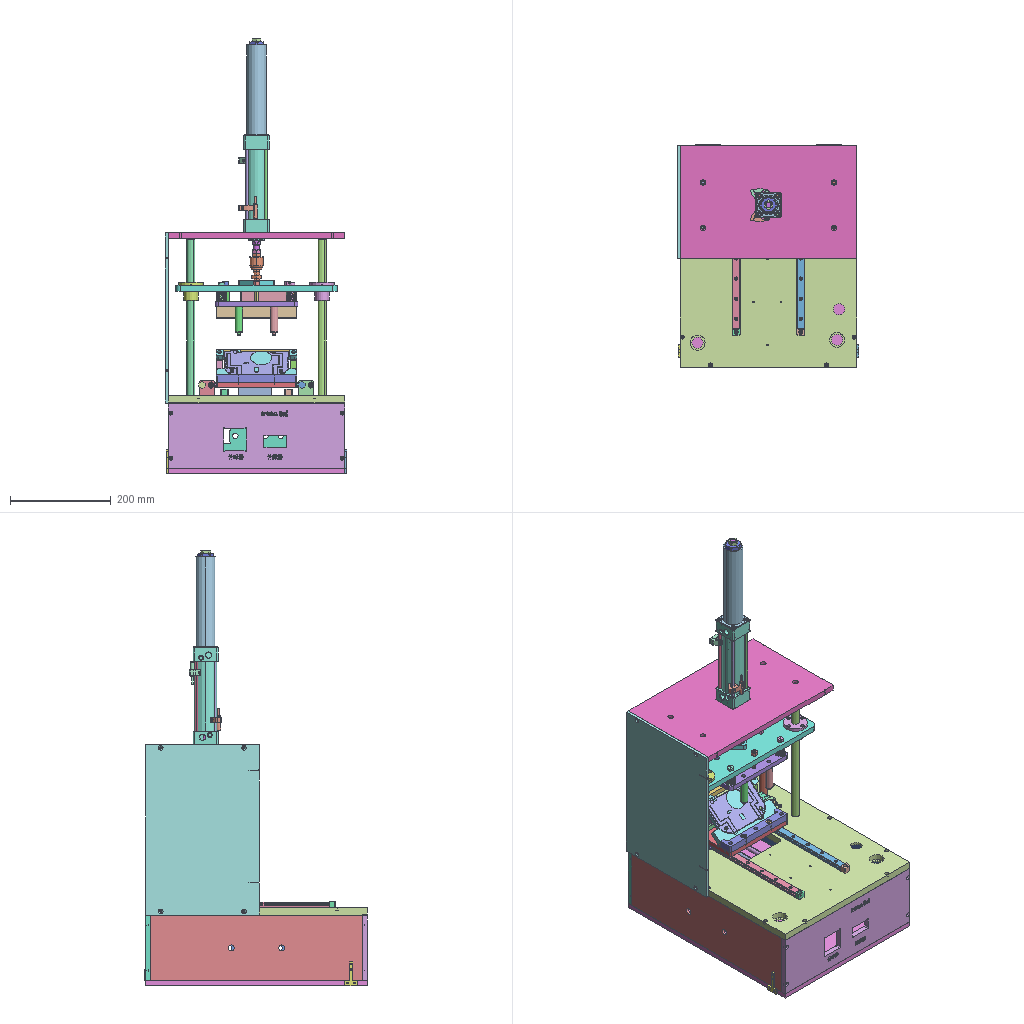Assembly | SolidWorks | 129 different items | 129 placed | box 360 x 442 x 864 mm
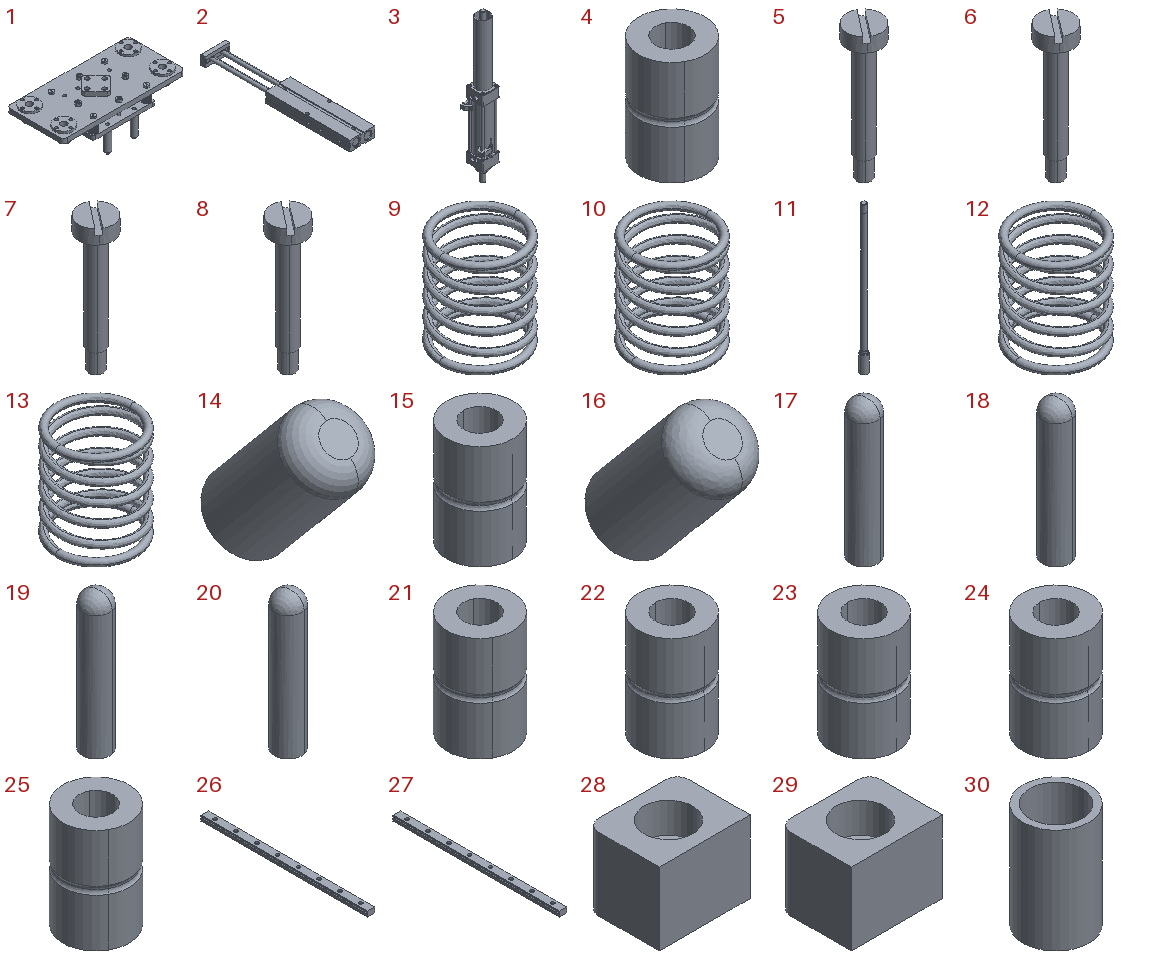Parts list (item | name | quantity | parent item | size | volume | features):
1 | (subassembly) | x1 | - | 320 x 150 x 110.25 mm | 967220 mm3 | -
2 | (subassembly) | x1 | - | 62.3 x 366.5 x 25.2 mm | 245376 mm3 | -
3 | (subassembly) | x1 | - | 59.782 x 64.739 x 435 mm | 326240 mm3 | -
4 | - | x1 | in 1 | 12 x 12 x 19 mm | 1601 mm3 | features BaseBody 1
5 | - | x1 | in 1 | 12 x 12 x 47 mm | 1645 mm3 | features BaseBody 1
6 | - | x1 | in 1 | 12 x 12 x 47 mm | 1645 mm3 | features BaseBody 1
7 | - | x1 | in 1 | 12 x 12 x 47 mm | 1645 mm3 | features BaseBody 1
8 | - | x1 | in 1 | 12 x 12 x 47 mm | 1645 mm3 | features BaseBody 1
9 | - | x1 | in 1 | 18.005 x 18.005 x 21.505 mm | 615.294 mm3 | features BaseBody 1
10 | - | x1 | in 1 | 18.005 x 18.005 x 21.505 mm | 615.294 mm3 | features BaseBody 1
11 | - | x1 | in 3 | 9 x 9 x 178.5 mm | 4474 mm3 | features BaseBody 1
12 | - | x1 | in 1 | 18.005 x 18.005 x 21.505 mm | 615.294 mm3 | features BaseBody 1
13 | - | x1 | in 1 | 18.005 x 18.005 x 21.505 mm | 615.294 mm3 | features BaseBody 1
14 | - | x1 | - | 6.9 x 12.824 x 13.576 mm | 469.908 mm3 | features BaseBody 1
15 | - | x1 | - | 12 x 12 x 19 mm | 1601 mm3 | features BaseBody 1
16 | - | x1 | - | 6.9 x 12.824 x 13.576 mm | 469.899 mm3 | features BaseBody 1
17 | - | x1 | in 1 | 6 x 6 x 30 mm | 732.824 mm3 | features BaseBody 1
18 | - | x1 | in 1 | 6 x 6 x 30 mm | 732.824 mm3 | features BaseBody 1
19 | - | x1 | in 1 | 6 x 6 x 30 mm | 732.824 mm3 | features BaseBody 1
20 | - | x1 | in 1 | 6 x 6 x 30 mm | 732.824 mm3 | features BaseBody 1
21 | - | x1 | in 1 | 12 x 12 x 19 mm | 1601 mm3 | features BaseBody 1
22 | - | x1 | - | 12 x 12 x 19 mm | 1601 mm3 | features BaseBody 1
23 | - | x1 | - | 12 x 12 x 19 mm | 1601 mm3 | features BaseBody 1
24 | - | x1 | - | 12 x 12 x 19 mm | 1601 mm3 | features BaseBody 1
25 | - | x1 | in 1 | 12 x 12 x 19 mm | 1601 mm3 | features BaseBody 1
26 | - | x1 | - | 15 x 320 x 10 mm | 44223 mm3 | features BaseBody 1
27 | - | x1 | - | 15 x 320 x 10 mm | 44223 mm3 | features BaseBody 1
28 | - | x1 | - | 15 x 12 x 12 mm | 1791 mm3 | features BaseBody 1
29 | - | x1 | - | 15 x 12 x 12 mm | 1791 mm3 | features BaseBody 1
30 | - | x1 | in 3 | 25 x 25 x 40 mm | 7069 mm3 | features BaseBody 1
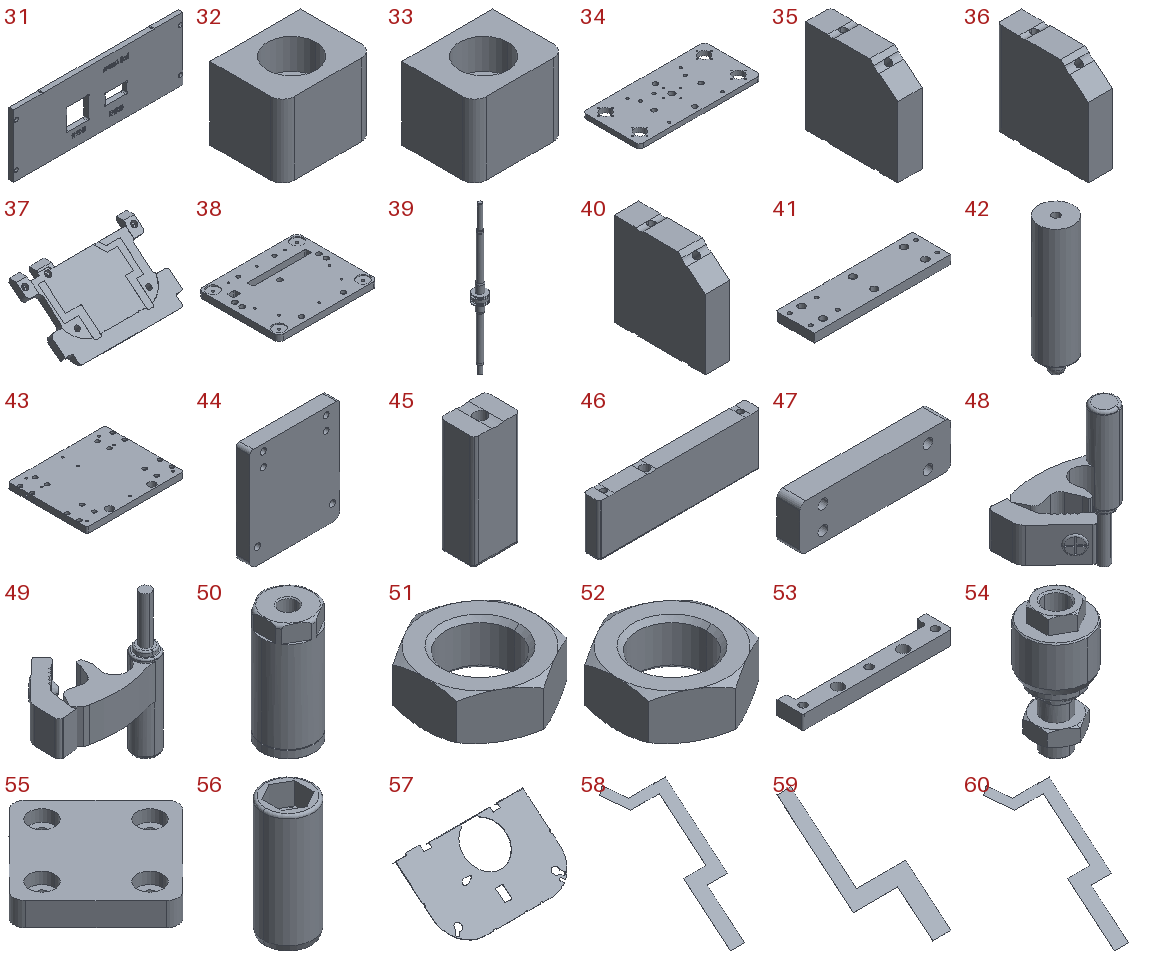31 | - | x1 | - | 350 x 10 x 130 mm | 422656 mm3 | features BaseBody 1, HoleWzd 1, ICE 1
32 | - | x1 | - | 15 x 12 x 12 mm | 1791 mm3 | features BaseBody 1
33 | - | x1 | - | 15 x 12 x 12 mm | 1791 mm3 | features BaseBody 1
34 | - | x1 | in 1 | 320 x 150 x 12 mm | 530945 mm3 | features BaseBody 1
35 | - | x1 | - | 12 x 45 x 45.902 mm | 23229 mm3 | features BaseBody 1
36 | - | x1 | - | 12 x 45 x 45.902 mm | 23224 mm3 | features BaseBody 1
37 | - | x1 | - | 160 x 86.9 x 65.902 mm | 123338 mm3 | features BaseBody 1
38 | - | x1 | in 1 | 164 x 134 x 10 mm | 201088 mm3 | features BaseBody 1
39 | - | x1 | in 3 | 39.5 x 39.5 x 435 mm | 104659 mm3 | features BaseBody 1
40 | - | x1 | - | 12 x 45 x 45.902 mm | 23264 mm3 | features BaseBody 1
41 | - | x1 | - | 160 x 45 x 10 mm | 67785 mm3 | features BaseBody 1
42 | - | x1 | in 1 | 15 x 15 x 59 mm | 9190 mm3 | features BaseBody 1, HoleWzd 1, MoveFace 1
43 | - | x1 | - | 160 x 130 x 10 mm | 201415 mm3 | features BaseBody 1
44 | - | x1 | - | 66 x 10 x 75.35 mm | 47694 mm3 | features BaseBody 1
45 | - | x1 | in 1 | 12.534 x 9.6 x 31.25 mm | 3446 mm3 | features BaseBody 1
46 | - | x1 | in 1 | 97.4 x 9.6 x 31.25 mm | 28550 mm3 | features BaseBody 1
47 | - | x1 | - | 66 x 10 x 19.75 mm | 12427 mm3 | features BaseBody 1
48 | - | x1 | in 3 | 36.145 x 22.709 x 44.1 mm | 4669 mm3 | features BaseBody 1
49 | - | x1 | in 3 | 36.145 x 22.709 x 44.1 mm | 4669 mm3 | features BaseBody 1
50 | - | x1 | - | 32 x 32 x 71 mm | 42303 mm3 | features BaseBody 1
51 | - | x1 | - | 17 x 19.63 x 7 mm | 1102 mm3 | features BaseBody 1
52 | - | x1 | - | 17 x 19.63 x 7 mm | 1102 mm3 | features BaseBody 1
53 | - | x1 | - | 160 x 28 x 15 mm | 41591 mm3 | features BaseBody 1, HoleWzd 1, MoveFace 1
54 | - | x1 | - | 28 x 28 x 58 mm | 19286 mm3 | features BaseBody 1
55 | - | x1 | in 1 | 70 x 70 x 10 mm | 24895 mm3 | features BaseBody 1
56 | - | x1 | in 3 | 9 x 9 x 21.5 mm | 900.711 mm3 | features BaseBody 1
57 | - | x1 | - | 127.4 x 62.108 x 51.15 mm | 3262 mm3 | features BaseBody 1
58 | - | x1 | - | 27.714 x 55.483 x 46.567 mm | 28.639 mm3 | features BaseBody 1
59 | - | x1 | - | 27.548 x 48.792 x 40.953 mm | 27.56 mm3 | features BaseBody 1
60 | - | x1 | - | 27.714 x 55.483 x 46.567 mm | 28.639 mm3 | features BaseBody 1
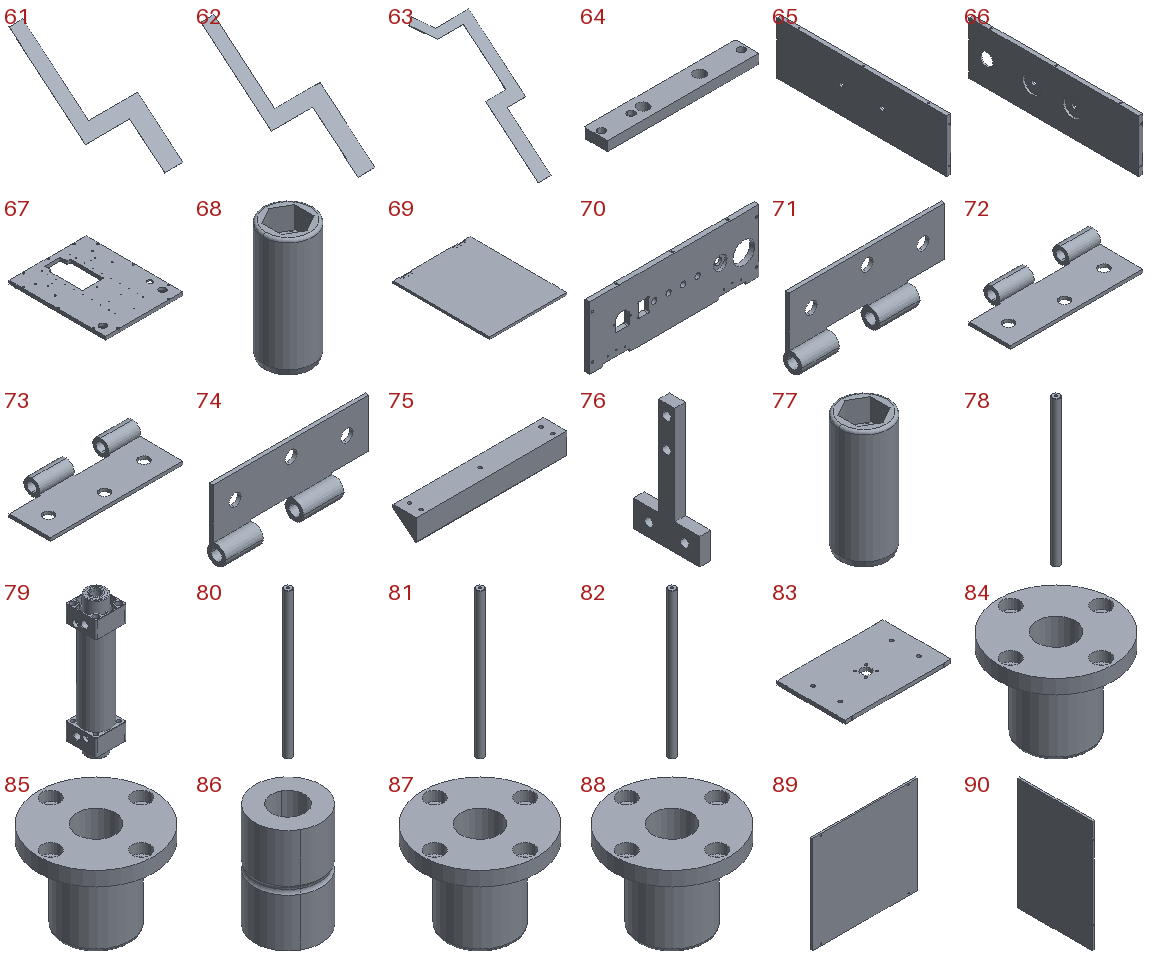61 | - | x1 | - | 27.548 x 48.792 x 40.953 mm | 27.56 mm3 | features BaseBody 1
62 | - | x1 | - | 27.548 x 54.936 x 46.114 mm | 46.14 mm3 | features BaseBody 1
63 | - | x1 | - | 27.714 x 60.861 x 51.086 mm | 46.633 mm3 | features BaseBody 1
64 | - | x1 | - | 160 x 25 x 10 mm | 36749 mm3 | features BaseBody 1, HoleWzd 1, MoveFace 1
65 | - | x1 | - | 10 x 420 x 130 mm | 527833 mm3 | features BaseBody 1
66 | - | x1 | - | 10 x 420 x 130 mm | 507586 mm3 | features BaseBody 1
67 | - | x1 | - | 350.001 x 440 x 15 mm | 1979972 mm3 | features BaseBody 1
68 | - | x1 | in 3 | 9 x 9 x 21.5 mm | 900.711 mm3 | features BaseBody 1
69 | - | x1 | - | 350 x 440 x 10 mm | 1538465 mm3 | features BaseBody 1
70 | - | x1 | - | 350 x 10 x 130 mm | 408343 mm3 | features BaseBody 1
71 | - | x1 | - | 50 x 6 x 22 mm | 1387 mm3 | features BaseBody 1
72 | - | x1 | - | 50 x 22 x 6 mm | 1387 mm3 | features BaseBody 1
73 | - | x1 | - | 50 x 22 x 6 mm | 1387 mm3 | features BaseBody 1
74 | - | x1 | - | 50 x 6 x 22 mm | 1387 mm3 | features BaseBody 1
75 | - | x1 | in 1 | 160 x 25 x 23.134 mm | 54327 mm3 | features BaseBody 1, DelFace 1
76 | - | x1 | - | 4 x 25 x 47 mm | 1759 mm3 | features BaseBody 1
77 | - | x1 | in 3 | 9 x 9 x 21.5 mm | 900.711 mm3 | features BaseBody 1
78 | - | x1 | - | 16 x 16 x 310 mm | 61335 mm3 | features BaseBody 1
79 | - | x1 | in 3 | 50 x 50 x 224 mm | 150469 mm3 | features BaseBody 1
80 | - | x1 | - | 16 x 16 x 310 mm | 61335 mm3 | features BaseBody 1
81 | - | x1 | - | 16 x 16 x 310 mm | 61335 mm3 | features BaseBody 1
82 | - | x1 | - | 16 x 16 x 310 mm | 61335 mm3 | features BaseBody 1
83 | - | x1 | - | 350 x 225 x 12 mm | 928615 mm3 | features BaseBody 1
84 | - | x1 | in 1 | 48 x 48 x 37 mm | 21560 mm3 | features BaseBody 1
85 | - | x1 | in 1 | 48 x 48 x 37 mm | 21560 mm3 | features BaseBody 1
86 | - | x1 | in 1 | 12 x 12 x 19 mm | 1601 mm3 | features BaseBody 1, DelFace 1
87 | - | x1 | in 1 | 48 x 48 x 37 mm | 21560 mm3 | features BaseBody 1
88 | - | x1 | in 1 | 48 x 48 x 37 mm | 21560 mm3 | features BaseBody 1
89 | - | x1 | - | 362 x 6 x 337.5 mm | 732487 mm3 | features BaseBody 1
90 | - | x1 | - | 6 x 225 x 337.5 mm | 454718 mm3 | features BaseBody 1
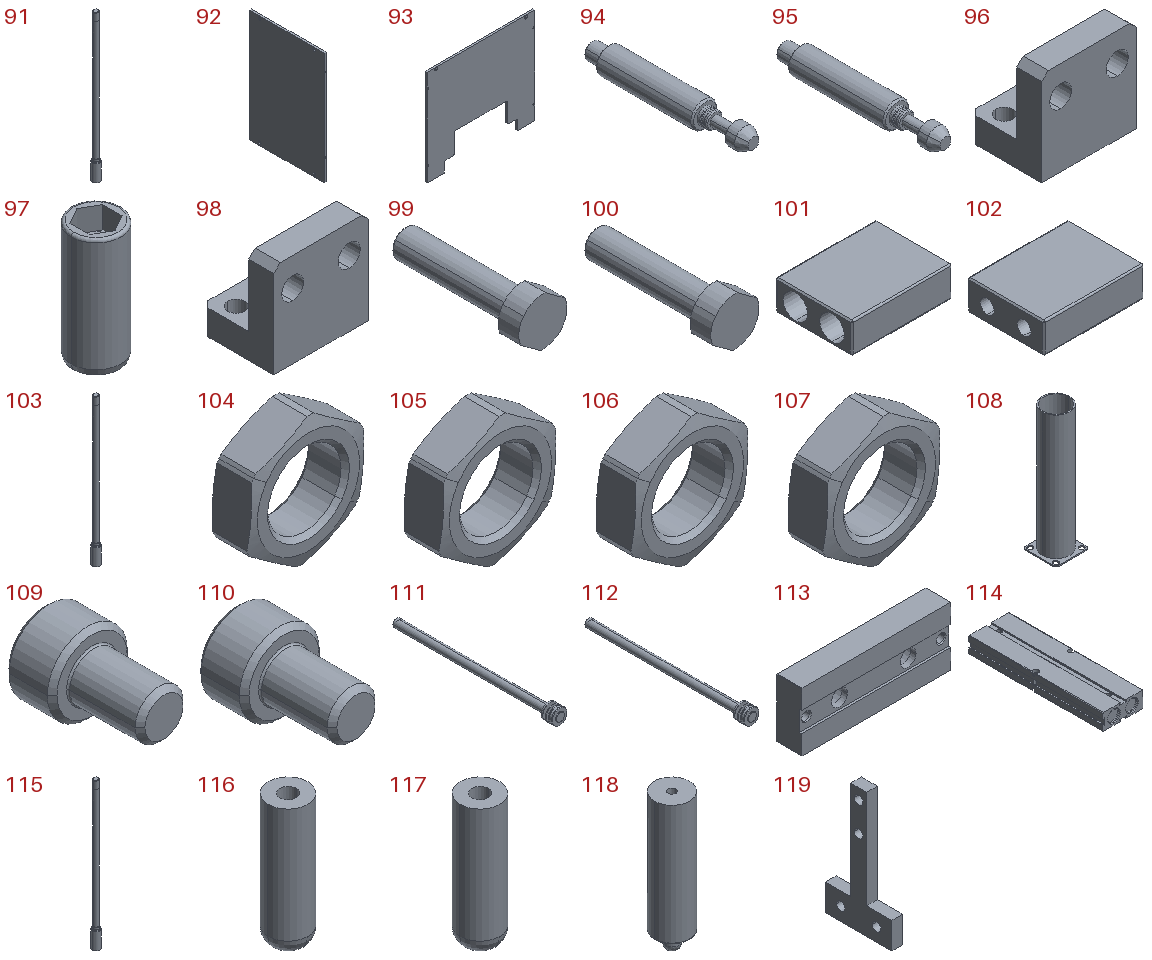91 | - | x1 | in 3 | 9 x 9 x 178.5 mm | 4474 mm3 | features BaseBody 1
92 | - | x1 | - | 6 x 224.9 x 337.5 mm | 454534 mm3 | features BaseBody 1
93 | - | x1 | - | 362 x 6 x 322.5 mm | 572741 mm3 | features BaseBody 1
94 | - | x1 | - | 8.001 x 50 x 8 mm | 1845 mm3 | features BaseBody 1
95 | - | x1 | - | 8.001 x 50 x 8 mm | 1845 mm3 | features BaseBody 1
96 | - | x1 | - | 30.001 x 23.001 x 30 mm | 9740 mm3 | features BaseBody 1
97 | - | x1 | in 3 | 9 x 9 x 21.5 mm | 900.711 mm3 | features BaseBody 1
98 | - | x1 | - | 30.001 x 23.001 x 30 mm | 9740 mm3 | features BaseBody 1
99 | - | x1 | - | 14 x 40 x 14 mm | 2585 mm3 | features BaseBody 1
100 | - | x1 | - | 14 x 40.001 x 14 mm | 2585 mm3 | features BaseBody 1
101 | - | x1 | - | 33 x 25 x 10 mm | 5939 mm3 | features BaseBody 1
102 | - | x1 | - | 33 x 25 x 10 mm | 5939 mm3 | features BaseBody 1
103 | - | x1 | in 3 | 9 x 9 x 178.5 mm | 4474 mm3 | features BaseBody 1
104 | - | x1 | - | 11.414 x 4 x 12.321 mm | 245.502 mm3 | features BaseBody 1
105 | - | x1 | - | 11.414 x 4.001 x 12.321 mm | 245.502 mm3 | features BaseBody 1
106 | - | x1 | - | 11.414 x 4 x 12.321 mm | 245.502 mm3 | features BaseBody 1
107 | - | x1 | - | 11.414 x 4.001 x 12.321 mm | 245.502 mm3 | features BaseBody 1
108 | - | x1 | in 3 | 48 x 48 x 180 mm | 33210 mm3 | features BaseBody 1
109 | - | x1 | - | 10 x 15 x 10 mm | 646.757 mm3 | features BaseBody 1
110 | - | x1 | - | 10 x 15 x 10 mm | 646.757 mm3 | features BaseBody 1
111 | - | x1 | in 2 | 19.6 x 212.6 x 19.6 mm | 18401 mm3 | features BaseBody 1
112 | - | x1 | in 2 | 19.6 x 212.6 x 19.6 mm | 18401 mm3 | features BaseBody 1
113 | - | x1 | in 2 | 61 x 10 x 24 mm | 12443 mm3 | features BaseBody 1
114 | - | x1 | in 2 | 62.3 x 217.5 x 25.2 mm | 196132 mm3 | features BaseBody 1
115 | - | x1 | in 3 | 9 x 9 x 178.5 mm | 4474 mm3 | features BaseBody 1
116 | - | x1 | in 1 | 6 x 6 x 20 mm | 493.517 mm3 | features BaseBody 1
117 | - | x1 | in 1 | 6 x 6 x 20 mm | 493.517 mm3 | features BaseBody 1
118 | - | x1 | in 1 | 15 x 15 x 59 mm | 9171 mm3 | features BaseBody 1
119 | - | x1 | - | 4 x 25 x 47 mm | 1759 mm3 | features BaseBody 1
120 | Bending Fixture 6 cell.sldasm-Part-38 (subassembly) | x1 | - | - | - | -
121 | Bending Fixture 6 cell.sldasm-Part-39 (subassembly) | x1 | - | - | - | -
122 | Bending Fixture 6 cell.sldasm-Part-40 (subassembly) | x1 | - | - | - | -
123 | Bending Fixture 6 cell.sldasm-Part-41 (subassembly) | x1 | - | - | - | -
124 | Bending Fixture 6 cell.sldasm-Part-42 (subassembly) | x1 | - | - | - | -
125 | Bending Fixture 6 cell.sldasm-Part-43 (subassembly) | x1 | - | - | - | -
126 | Bending Fixture 6 cell.sldasm-Part-44 (subassembly) | x1 | - | - | - | -
127 | Bending Fixture 6 cell.sldasm-Part-45 (subassembly) | x1 | - | - | - | -
128 | Bending Fixture 6 cell.sldasm-Part-46 (subassembly) | x1 | - | - | - | -
129 | Bending Fixture 6 cell.sldasm-Part-47 (subassembly) | x1 | - | - | - | -